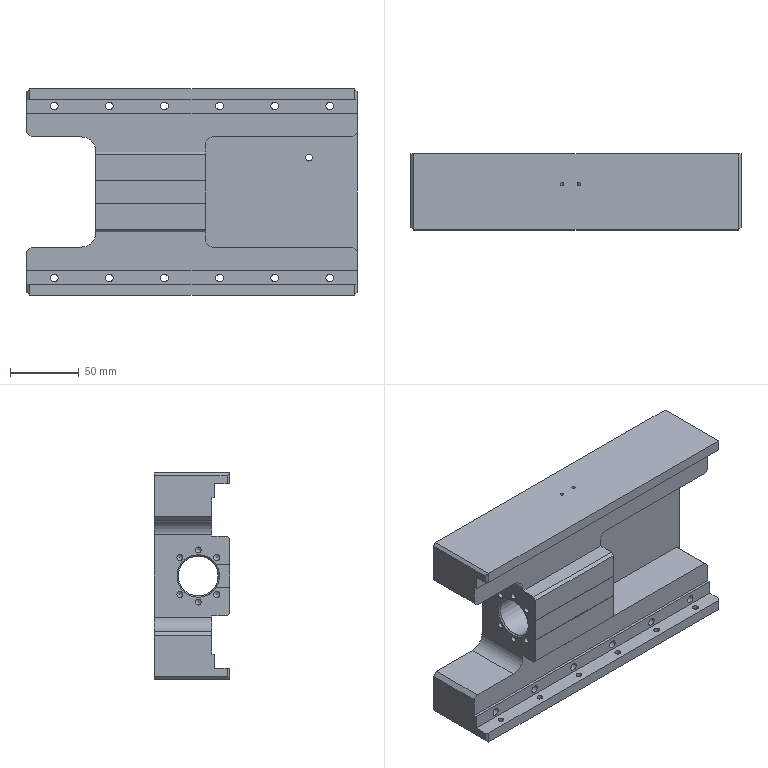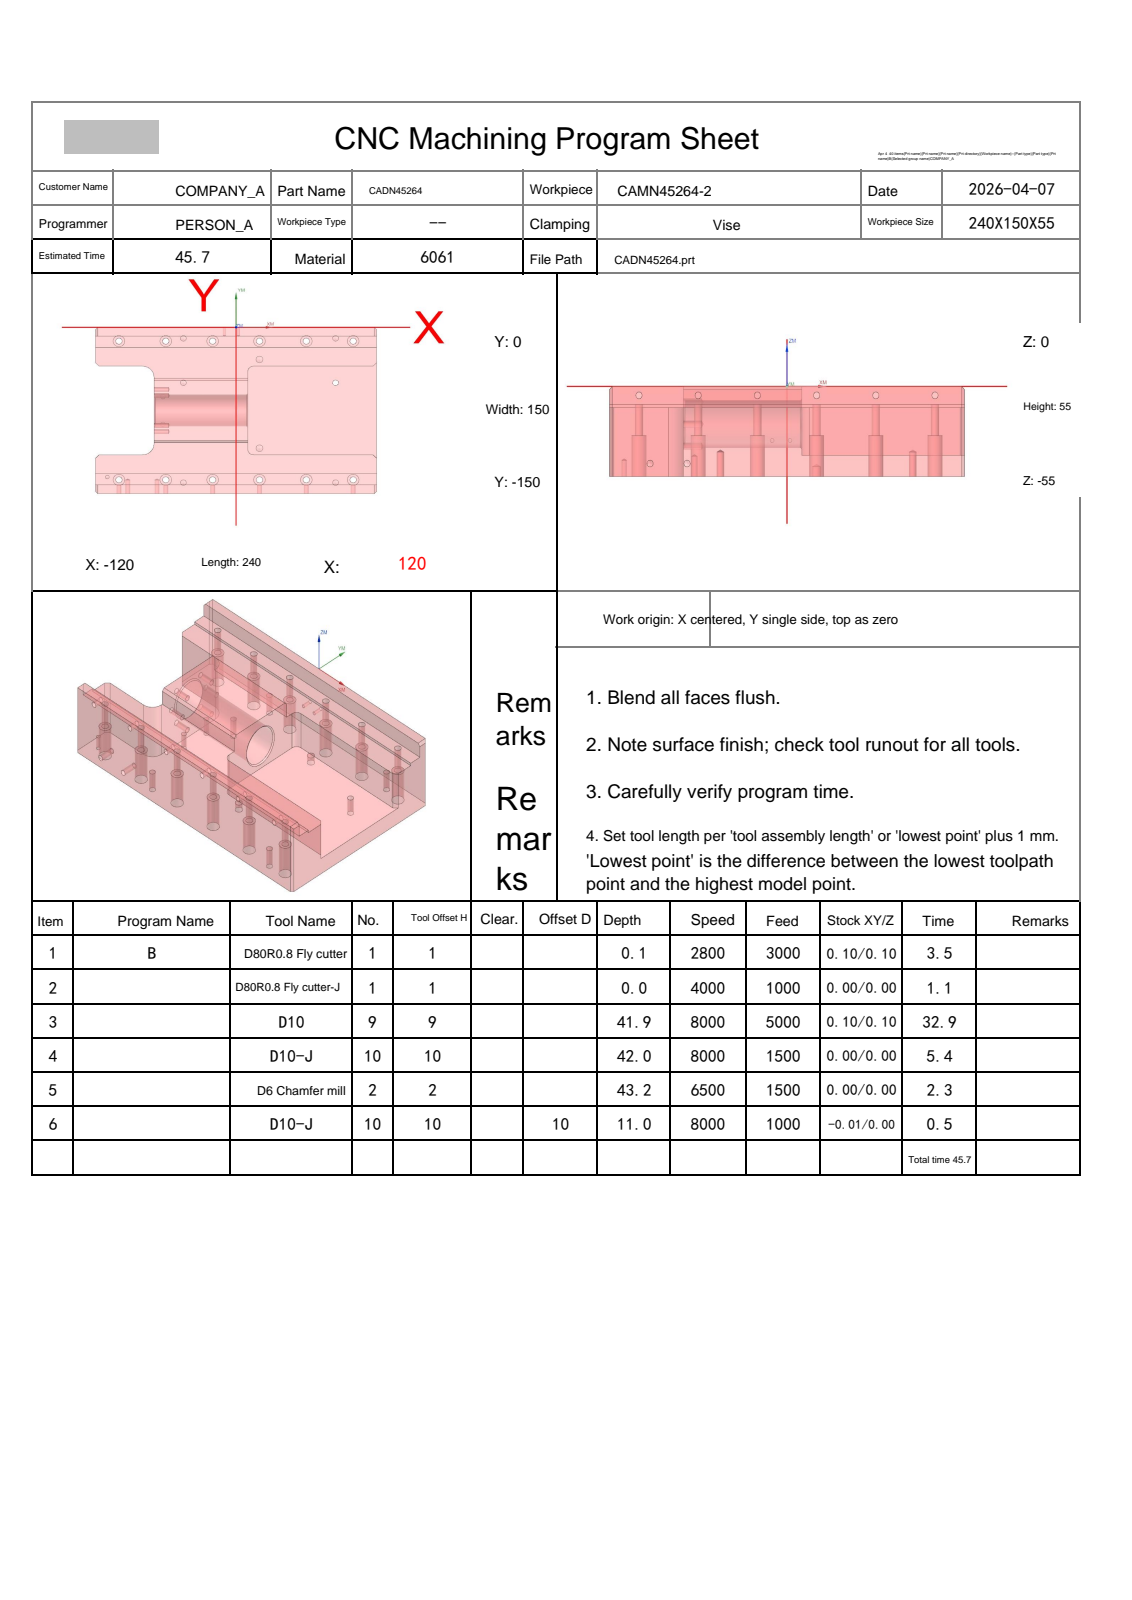NC program | NX | posted by the shop | part box 240 x 55 x 150 mm
Lines 209 to 1333 of 15848:
N3 T09 M06
(D10  D=10. R=0. H=09 ce=0.10 di=0.10)
G00 G90 G54 X134.5 Y-68. M03 S8000
G43 H09 Z14.5
M08
Z.626
G01 Z-.574 F5000.
X127.08
G03 X120.08 Y-75. I0.0 J-7.
G01 Y-110.836
X120.213 Y-110.937
X120.692 Y-111.365
X123. Y-113.672
Y-115.112
X120.08 Y-118.033
Y-126.698
Y-127.517
Y-136.418
Y-136.823
G02 X124.225 Y-139.047 I-.107 J-5.175
X125.085 Y-141.392 I-5.384 J-3.303
X125.115 Y-142. I-6.49 J-.629
G01 Y-148.068
X123.714 Y-149.47
X123.715 Y-142.
G03 X118.594 Y-136.9 I-5.121 J-.021
G01 X118.574
X-118.574
X-118.594
G03 X-123.715 Y-142. I0.0 J-5.121
G01 X-123.714 Y-149.467
X-125.115 Y-148.059
Y-141.994
G02 X-125.039 Y-141.028 I6.521 J-.026
X-123. Y-137.826 I5.116 J-1.008
X-120.08 Y-136.824 I3.077 J-4.21
G01 Y-136.418
Y-127.517
Y-126.698
Y-118.
X-120.057 Y-117.943
X-117.057 Y-114.943
X-117. Y-114.92
X-80.424
X-79.534 Y-114.909
X-78.648 Y-114.827
X-77.761 Y-114.664
X-76.874 Y-114.414
X-76.45 Y-114.263
X-75.989 Y-114.073
X-75.102 Y-113.626
X-74.43 Y-113.208
X-74.217 Y-113.06
X-73.329 Y-112.342
X-72.442 Y-111.425
X-72.102 Y-111.002
X-71.784 Y-110.56
X-71.556 Y-110.207
X-71.252 Y-109.677
X-70.925 Y-109.005
X-70.911 Y-108.936
X-70.845 Y-108.961
X-70.458 Y-108.999
X-70.082 Y-109.018
X-70.08 Y-107.714
X-65.641 Y-107.715
X10.
G03 X15.1 Y-102.574 I-.057 J5.157
G01 Y-47.426
G03 X10. Y-42.285 I-5.157 J-.015
G01 X-65.658
X-70.08 Y-42.286
X-70.082 Y-40.982
X-70.456 Y-41.001
X-70.826 Y-41.048
X-70.892 Y-41.075
X-70.907 Y-41.005
X-71.252 Y-40.323
X-71.556 Y-39.793
X-71.784 Y-39.441
X-72.457 Y-38.557
X-73.329 Y-37.658
X-74.217 Y-36.94
X-74.43 Y-36.792
X-75.101 Y-36.374
X-76.033 Y-35.908
X-76.875 Y-35.585
X-77.761 Y-35.336
X-78.648 Y-35.173
X-79.534 Y-35.091
X-80.424 Y-35.08
X-117.
X-117.057 Y-35.057
X-120.057 Y-32.057
X-120.08 Y-32.
Y-23.302
Y-22.483
Y-13.582
Y-13.176
G02 X-125.039 Y-8.972 I.157 J5.212
X-125.115 Y-8. I6.445 J.993
G01 Y-1.932
X-123.714 Y-.53
X-123.715 Y-8.
G03 X-118.594 Y-13.1 I5.121 J.021
G01 X-118.574
X118.574
X118.594
G03 X123.715 Y-8. I0.0 J5.121
G01 X123.714 Y-.533
X125.115 Y-1.941
Y-8.006
G02 X125.04 Y-8.965 I-6.521 J.026
X120.08 Y-13.176 I-5.118 J1.002
G01 Y-13.582
Y-22.483
Y-23.302
Y-31.967
X123. Y-34.888
Y-36.328
X120.69 Y-38.637
X120.356 Y-38.947
X120.08 Y-39.164
Y-71.986
G02 X119.662 Y-72.799 I-1. J0.0
G01 X113.498 Y-77.201
G03 X113.08 Y-78.014 I.582 J-.813
G01 Y-110.836
G03 X113.83 Y-113.987 I7. J0.0
G02 X113.935 Y-114.434 I-.894 J-.447
X113.83 Y-114.881 I-1. J0.0
G03 X113.08 Y-118.033 I6.25 J-3.152
G01 Y-126.696
Y-127.516
Y-128.903
G02 X112.083 Y-129.9 I-1. J.003
G01 X-71.13
G02 X-71.83 Y-129.613 I0.0 J1.
G01 X-73.319 Y-128.152
G03 X-73.767 Y-127.898 I-.7 J-.714
G02 X-75.638 Y-125.478 I.629 J2.42
X-73.741 Y-123.052 I2.5 J0.0
G01 X-66.347 Y-121.217
G02 X-65.745 Y-121.143 I.602 J-2.426
X-63.245 Y-123.643 I0.0 J-2.5
X-65.143 Y-126.07 I-2.5 J0.0
G01 X-71.264 Y-127.589
G03 X-71.774 Y-127.899 I.241 J-.971
G01 X-73.235 Y-129.56
G02 X-73.986 Y-129.9 I-.751 J.66
G01 X-112.083
G02 X-113.08 Y-128.903 I.003 J1.
G01 Y-127.516
Y-126.696
Y-122.917
G02 X-112.083 Y-121.92 I1. J-.003
G01 X-80.381
X-79.17 Y-121.905
X-77.69 Y-121.769
X-76.176 Y-121.49
X-74.746 Y-121.088
X-73.936 Y-120.798
X-73.077 Y-120.444
X-71.673 Y-119.737
X-70.576 Y-119.055
X-70.007 Y-118.658
X-68.595 Y-117.516
X-67.188 Y-116.061
X-66.526 Y-115.239
X-66.448 Y-115.129
G02 X-65.641 Y-114.715 I.811 J-.586
G01 X10.039
G03 X22.1 Y-102.584 I-.096 J12.157
G01 Y-47.416
G03 X10.039 Y-35.285 I-12.157 J-.026
G01 X-65.658
G02 X-66.448 Y-34.893 I.003 J1.
G01 X-67.141 Y-33.984
X-68.599 Y-32.481
X-70.007 Y-31.342
X-70.576 Y-30.945
X-71.68 Y-30.259
X-73.207 Y-29.494
X-74.67 Y-28.934
X-76.176 Y-28.51
X-77.69 Y-28.231
X-79.17 Y-28.095
X-80.381 Y-28.08
X-112.083
G02 X-113.08 Y-27.083 I.003 J1.
G01 Y-23.304
Y-22.484
Y-21.097
G02 X-112.083 Y-20.1 I1. J-.003
G01 X-73.995
G02 X-73.244 Y-20.44 I0.0 J-1.
G01 X-71.782 Y-22.101
G03 X-71.272 Y-22.412 I.751 J.66
G01 X-65.144 Y-23.929
G02 X-63.245 Y-26.355 I-.601 J-2.427
X-65.745 Y-28.855 I-2.5 J0.0
X-66.345 Y-28.782 I0.0 J2.5
G01 X-73.746 Y-26.95
G02 X-75.645 Y-24.523 I.601 J2.427
X-73.776 Y-22.104 I2.5 J0.0
G03 X-73.328 Y-21.85 I-.252 J.968
G01 X-71.838 Y-20.387
G02 X-71.137 Y-20.1 I.701 J-.713
G01 X112.083
G02 X113.08 Y-21.097 I-.003 J-1.
G01 Y-22.484
Y-23.304
Y-31.967
G03 X113.829 Y-35.118 I7. J0.0
G02 X113.935 Y-35.565 I-.895 J-.447
X113.829 Y-36.012 I-1. J0.0
G03 X113.08 Y-39.164 I6.251 J-3.151
G01 Y-71.986
G02 X112.662 Y-72.799 I-1. J0.0
G01 X106.498 Y-77.201
G03 X106.08 Y-78.014 I.582 J-.813
G01 Y-110.836
G03 X106.49 Y-114.198 I14. J0.0
G02 X106.518 Y-114.434 I-.972 J-.236
X106.49 Y-114.671 I-1. J0.0
G03 X106.08 Y-118.033 I13.59 J-3.362
G01 Y-121.904
G02 X105.084 Y-122.9 I-1. J.004
G01 X28.712
G02 X28.047 Y-122.647 I0.0 J1.
G01 X26.93 Y-121.653
G03 X26.311 Y-121.401 I-.664 J-.747
G02 X23.923 Y-118.904 I.112 J2.497
X25.377 Y-116.633 I2.5 J0.0
G01 X30.003 Y-114.503
G02 X31.049 Y-114.274 I1.046 J-2.271
X33.549 Y-116.774 I0.0 J-2.5
X32.095 Y-119.044 I-2.5 J0.0
G01 X28.471 Y-120.713
G03 X28.104 Y-121.002 I.418 J-.908
G01 X26.907 Y-122.519
G02 X26.122 Y-122.9 I-.785 J.619
G01 X-62.888
G02 X-63.385 Y-122.4 I.003 J.5
X-63.246 Y-122.054 I.5 J0.0
G01 X-63.063 Y-121.865
G02 X-62.709 Y-121.715 I.357 J-.35
G01 X10.066
G03 X29.1 Y-102.591 I-.123 J19.157
G01 Y-47.409
G03 X10.066 Y-28.285 I-19.157 J-.033
G01 X-62.708
G02 X-63.062 Y-28.135 I.003 J.5
G01 X-63.246 Y-27.946
G02 X-63.385 Y-27.6 I.361 J.346
X-62.887 Y-27.1 I.5 J0.0
G01 X26.122
G02 X26.907 Y-27.481 I0.0 J-1.
G01 X28.104 Y-28.998
G03 X28.47 Y-29.286 I.785 J.62
G01 X32.095 Y-30.956
G02 X33.549 Y-33.226 I-1.046 J-2.271
X31.049 Y-35.726 I-2.5 J0.0
X30.003 Y-35.497 I0.0 J2.5
G01 X25.377 Y-33.367
G02 X23.923 Y-31.096 I1.046 J2.271
X26.311 Y-28.599 I2.5 J0.0
G03 X26.93 Y-28.347 I-.045 J.999
G01 X28.047 Y-27.353
G02 X28.712 Y-27.1 I.665 J-.747
G01 X105.084
G02 X106.08 Y-28.096 I-.004 J-1.
G01 Y-31.967
G03 X106.49 Y-35.329 I14. J0.0
G02 X106.518 Y-35.565 I-.972 J-.236
X106.49 Y-35.801 I-1. J0.0
G03 X106.08 Y-39.164 I13.59 J-3.362
G01 Y-71.986
G02 X105.662 Y-72.799 I-1. J0.0
G01 X99.498 Y-77.201
G03 X99.08 Y-78.014 I.582 J-.813
G01 Y-110.836
G03 X99.364 Y-114.275 I21. J0.0
G01 X99.376 Y-114.434
X99.364 Y-114.594
G03 X99.293 Y-115.047 I20.716 J-3.439
G02 X98.309 Y-115.9 I-.989 J.147
G01 X34.129
G02 X33.134 Y-114.9 I.005 J1.
X33.241 Y-114.45 I1. J0.0
G03 X36.1 Y-102.597 I-23.298 J11.891
G01 Y-47.403
G03 X33.241 Y-35.55 I-26.157 J-.039
G02 X33.134 Y-35.1 I.893 J.45
X34.129 Y-34.1 I1. J0.0
G01 X98.309
G02 X99.293 Y-34.953 I-.005 J-1.
G03 X99.364 Y-35.406 I20.787 J2.986
G01 X99.376 Y-35.565
X99.364 Y-35.724
G03 X99.08 Y-39.164 I20.716 J-3.439
G01 Y-71.986
G02 X98.662 Y-72.799 I-1. J0.0
G01 X92.498 Y-77.201
G03 X92.08 Y-78.014 I.582 J-.813
G01 Y-107.905
G02 X91.085 Y-108.9 I-1. J.005
G01 X43.675
G02 X42.68 Y-107.9 I.005 J1.
G01 X42.691 Y-107.748
G03 X43.1 Y-102.603 I-32.748 J5.19
G01 Y-47.397
G03 X42.691 Y-42.252 I-33.157 J-.044
G01 X42.68 Y-42.1
G02 X43.675 Y-41.1 I1. J0.0
G01 X91.085
G02 X92.08 Y-42.095 I-.005 J-1.
G01 Y-71.986
G02 X91.662 Y-72.799 I-1. J0.0
G01 X85.498 Y-77.201
G03 X85.08 Y-78.014 I.582 J-.813
G01 Y-100.905
G02 X84.085 Y-101.9 I-1. J.005
G01 X51.095
G02 X50.1 Y-100.905 I.005 J1.
G01 Y-49.095
G02 X51.095 Y-48.1 I1. J-.005
G01 X84.085
G02 X85.08 Y-49.095 I-.005 J-1.
G01 Y-71.986
G02 X84.662 Y-72.799 I-1. J0.0
G01 X78.498 Y-77.201
G03 X78.08 Y-78.014 I.582 J-.813
G01 Y-93.905
G02 X77.085 Y-94.9 I-1. J.005
G01 X58.095
G02 X57.1 Y-93.905 I.005 J1.
G01 Y-56.095
G02 X58.095 Y-55.1 I1. J-.005
G01 X77.085
G02 X78.08 Y-56.095 I-.005 J-1.
G01 Y-71.986
G02 X77.662 Y-72.799 I-1. J0.0
G01 X71.498 Y-77.201
G03 X71.08 Y-78.014 I.582 J-.814
G01 Y-86.905
G02 X70.085 Y-87.9 I-1. J.005
G01 X65.095
G02 X64.1 Y-86.905 I.005 J1.
G01 Y-63.095
G02 X65.095 Y-62.1 I1. J-.005
G01 X70.085
G02 X71.08 Y-63.095 I-.005 J-1.
G01 Y-75.
Y-75.5
G03 X78.08 Y-82.5 I7. J0.0
G01 Z.626
G00 Z3.
G01 X134.5 Y-68. F6000.
G00 Z.053
G01 Z-1.147 F5000.
X127.08
G03 X120.08 Y-75. I0.0 J-7.
G01 Y-110.836
X120.213 Y-110.937
X120.692 Y-111.365
X123. Y-113.672
Y-115.112
X120.08 Y-118.033
Y-126.698
Y-127.517
Y-135.565
Y-136.418
Y-136.823
G02 X124.225 Y-139.047 I-.107 J-5.175
X125.158 Y-142.35 I-5.384 J-3.303
X125.151 Y-142.651 I-6.317 J0.0
G01 Y-148.
X125.127 Y-148.056
X124.287 Y-148.896
X124.289 Y-142.
G03 X119.158 Y-136.9 I-5.131 J-.031
G01 X119.147
X-119.147
X-119.158
G03 X-124.289 Y-142. I0.0 J-5.131
G01 X-124.287 Y-148.891
X-125.127 Y-148.046
X-125.151 Y-147.99
Y-142.647
X-125.13 Y-141.755
G02 X-120.08 Y-136.824 I5.207 J-.281
G01 Y-136.418
Y-135.565
Y-127.517
Y-126.698
Y-118.
X-120.057 Y-117.943
X-117.057 Y-114.943
X-117. Y-114.92
X-80.424
X-79.534 Y-114.909
X-78.648 Y-114.827
X-77.761 Y-114.664
X-76.874 Y-114.414
X-76.45 Y-114.263
X-75.989 Y-114.073
X-75.102 Y-113.626
X-74.43 Y-113.208
X-74.217 Y-113.06
X-73.329 Y-112.342
X-72.442 Y-111.425
X-72.102 Y-111.002
X-71.784 Y-110.56
X-71.556 Y-110.207
X-71.252 Y-109.677
X-70.925 Y-109.005
X-70.911 Y-108.936
X-70.845 Y-108.961
X-70.458 Y-108.999
X-70.082 Y-109.018
X-70.081 Y-108.287
X-66.091 Y-108.289
X10.063
G03 X13.404 Y-106.978 I0.0 J4.915
X15.1 Y-103.147 I-3.602 J3.886
G01 Y-46.853
X15.052 Y-46.317
G03 X10.011 Y-41.711 I-5.041 J-.456
G01 X-66.096
X-70.081 Y-41.713
Y-41.489
X-70.082 Y-40.982
X-70.456 Y-41.001
X-70.826 Y-41.048
X-70.892 Y-41.075
X-70.907 Y-41.005
X-71.252 Y-40.323
X-71.556 Y-39.793
X-71.784 Y-39.441
X-72.457 Y-38.557
X-73.329 Y-37.658
X-74.217 Y-36.94
X-74.43 Y-36.792
X-75.101 Y-36.374
X-76.033 Y-35.908
X-76.875 Y-35.585
X-77.761 Y-35.336
X-78.648 Y-35.173
X-79.534 Y-35.091
X-80.424 Y-35.08
X-117.
X-117.057 Y-35.057
X-120.057 Y-32.057
X-120.08 Y-32.
Y-23.302
Y-22.483
Y-14.435
Y-13.582
Y-13.176
G02 X-125.13 Y-8.242 I.157 J5.212
G01 X-125.151 Y-6.461
Y-2.
X-125.127 Y-1.944
X-124.287 Y-1.104
X-124.289 Y-8.
G03 X-119.158 Y-13.1 I5.131 J.031
G01 X-119.147
X119.147
X119.158
G03 X124.289 Y-8. I0.0 J5.131
G01 X124.287 Y-1.109
X125.127 Y-1.954
X125.151 Y-2.01
Y-6.462
X125.13 Y-8.245
G02 X123. Y-12.174 I-5.208 J.282
X120.08 Y-13.176 I-3.078 J4.21
G01 Y-13.582
Y-14.435
Y-22.483
Y-23.302
Y-31.967
X123. Y-34.888
Y-36.328
X120.69 Y-38.637
X120.356 Y-38.947
X120.08 Y-39.164
Y-71.986
G02 X119.662 Y-72.799 I-1. J0.0
G01 X113.498 Y-77.201
G03 X113.08 Y-78.014 I.582 J-.813
G01 Y-110.836
G03 X113.83 Y-113.988 I7. J0.0
G02 X113.935 Y-114.434 I-.895 J-.447
X113.83 Y-114.881 I-1. J0.0
G03 X113.08 Y-118.033 I6.25 J-3.152
G01 Y-126.696
Y-127.516
Y-128.904
G02 X112.083 Y-129.9 I-1. J.004
G01 X-71.135
G02 X-71.836 Y-129.613 I0.0 J1.
G01 X-73.33 Y-128.144
G03 X-73.776 Y-127.89 I-.701 J-.713
G02 X-75.64 Y-125.472 I.636 J2.418
X-73.736 Y-123.044 I2.5 J0.0
G01 X-66.641 Y-121.303
G02 X-66.045 Y-121.231 I.596 J-2.428
X-63.545 Y-123.731 I0.0 J-2.5
X-65.449 Y-126.159 I-2.5 J0.0
G01 X-71.268 Y-127.587
G03 X-71.78 Y-127.897 I.238 J-.971
G01 X-73.245 Y-129.561
G02 X-73.996 Y-129.9 I-.75 J.661
G01 X-112.083
G02 X-113.08 Y-128.904 I.004 J1.
G01 Y-127.516
Y-126.696
Y-122.916
G02 X-112.084 Y-121.92 I1. J-.004
G01 X-80.381
X-79.17 Y-121.905
X-77.69 Y-121.769
X-76.176 Y-121.49
X-74.746 Y-121.088
X-73.936 Y-120.798
X-73.077 Y-120.444
X-71.673 Y-119.737
X-70.576 Y-119.055
X-70.007 Y-118.658
X-68.59 Y-117.511
X-67.188 Y-116.061
X-66.864 Y-115.659
G02 X-66.091 Y-115.289 I.777 J-.629
G01 X10.063
G03 X18.163 Y-112.112 I0.0 J11.915
X22.1 Y-103.184 I-8.361 J9.019
G01 X22.023 Y-45.687
G03 X10.011 Y-34.711 I-12.012 J-1.086
G01 X-66.096
G02 X-66.885 Y-34.32 I.004 J1.
G01 X-67.141 Y-33.984
X-68.599 Y-32.481
X-70.007 Y-31.342
X-70.576 Y-30.945
X-71.68 Y-30.259
X-73.207 Y-29.494
X-74.67 Y-28.934
X-76.176 Y-28.51
X-77.69 Y-28.231
X-79.17 Y-28.095
X-80.381 Y-28.08
X-112.084
G02 X-113.08 Y-27.084 I.004 J1.
G01 Y-23.304
Y-22.484
Y-21.096
G02 X-112.083 Y-20.1 I1. J-.004
G01 X-74.005
G02 X-73.254 Y-20.439 I0.0 J-1.
G01 X-71.788 Y-22.103
G03 X-71.276 Y-22.414 I.75 J.661
G01 X-65.451 Y-23.839
G02 X-63.545 Y-26.268 I-.594 J-2.428
X-66.045 Y-28.768 I-2.5 J0.0
X-66.639 Y-28.696 I0.0 J2.5
G01 X-73.741 Y-26.958
G02 X-75.647 Y-24.529 I.594 J2.428
X-73.785 Y-22.112 I2.5 J0.0
G03 X-73.339 Y-21.858 I-.255 J.967
G01 X-71.844 Y-20.387
G02 X-71.143 Y-20.1 I.701 J-.713
G01 X112.083
G02 X113.08 Y-21.096 I-.004 J-1.
G01 Y-22.484
Y-23.304
Y-31.967
G03 X113.83 Y-35.119 I7. J0.0
G02 X113.935 Y-35.565 I-.895 J-.447
X113.83 Y-36.012 I-1. J0.0
G03 X113.08 Y-39.164 I6.25 J-3.152
G01 Y-71.986
G02 X112.662 Y-72.799 I-1. J0.0
G01 X106.498 Y-77.201
G03 X106.08 Y-78.014 I.582 J-.813
G01 Y-110.836
G03 X106.49 Y-114.198 I14. J0.0
G02 X106.518 Y-114.434 I-.972 J-.236
X106.49 Y-114.67 I-1. J0.0
G03 X106.08 Y-118.033 I13.59 J-3.363
G01 Y-121.904
G02 X105.084 Y-122.9 I-1. J.004
G01 X29.213
G02 X28.551 Y-122.649 I0.0 J1.
G01 X27.459 Y-121.684
G03 X26.827 Y-121.434 I-.662 J-.75
G02 X24.402 Y-118.935 I.075 J2.499
X25.824 Y-116.68 I2.5 J0.0
G01 X30.273 Y-114.553
G02 X31.351 Y-114.308 I1.078 J-2.255
X33.851 Y-116.808 I0.0 J-2.5
X32.43 Y-119.063 I-2.5 J0.0
G01 X28.963 Y-120.721
G03 X28.607 Y-121.007 I.431 J-.902
G01 X27.426 Y-122.516
G02 X26.638 Y-122.9 I-.788 J.616
G01 X-63.359
G02 X-63.657 Y-122.599 I.003 J.301
X-63.56 Y-122.379 I.301 J0.0
X-63.348 Y-122.289 I.214 J-.21
G01 X10.063
G03 X22.922 Y-117.245 I0.0 J18.915
X29.1 Y-103.205 I-13.121 J14.152
G01 X29.023 Y-45.366
G03 X10.013 Y-27.711 I-19.009 J-1.406
G01 X10.011
X-63.349
G02 X-63.574 Y-27.607 I.002 J.301
X-63.657 Y-27.4 I.217 J.207
X-63.36 Y-27.1 I.3 J0.0
G01 X26.653
G02 X27.441 Y-27.484 I0.0 J-1.
G01 X28.622 Y-28.994
G03 X28.978 Y-29.279 I.787 J.617
G01 X32.443 Y-30.934
G02 X33.866 Y-33.19 I-1.077 J-2.256
X31.366 Y-35.69 I-2.5 J0.0
X30.288 Y-35.446 I0.0 J2.5
G01 X25.84 Y-33.322
G02 X24.418 Y-31.066 I1.077 J2.256
X26.842 Y-28.567 I2.5 J0.0
G03 X27.473 Y-28.317 I-.03 J1.
G01 X28.566 Y-27.351
G02 X29.229 Y-27.1 I.662 J-.749
G01 X105.084
G02 X106.08 Y-28.096 I-.004 J-1.
G01 Y-31.967
G03 X106.49 Y-35.329 I14. J0.0
G02 X106.518 Y-35.565 I-.972 J-.236
X106.49 Y-35.801 I-1. J0.0
G03 X106.08 Y-39.164 I13.59 J-3.362
G01 Y-71.986
G02 X105.662 Y-72.799 I-1. J0.0
G01 X99.498 Y-77.201
G03 X99.08 Y-78.014 I.582 J-.813
G01 Y-110.836
G03 X99.364 Y-114.275 I21. J0.0
G01 X99.376 Y-114.434
X99.364 Y-114.593
G03 X99.293 Y-115.047 I20.716 J-3.44
G02 X98.309 Y-115.9 I-.989 J.147
G01 X34.41
G02 X33.415 Y-114.9 I.005 J1.
X33.511 Y-114.472 I1. J0.0
G03 X36.1 Y-103.221 I-23.709 J11.379
G01 X36.022 Y-45.103
G03 X33.524 Y-35.527 I-26.008 J-1.673
G02 X33.428 Y-35.1 I.904 J.427
X34.423 Y-34.1 I1. J0.0
G01 X98.309
G02 X99.293 Y-34.953 I-.005 J-1.
G03 X99.364 Y-35.406 I20.787 J2.986
G01 X99.376 Y-35.565
X99.364 Y-35.724
G03 X99.08 Y-39.164 I20.716 J-3.439
G01 Y-71.986
G02 X98.662 Y-72.799 I-1. J0.0
G01 X92.498 Y-77.201
G03 X92.08 Y-78.014 I.582 J-.813
G01 Y-107.905
G02 X91.085 Y-108.9 I-1. J.005
G01 X43.757
G02 X42.762 Y-107.9 I.005 J1.
G01 X42.771 Y-107.765
G03 X43.1 Y-103.233 I-32.969 J4.672
G01 X43.022 Y-44.873
X43.008 Y-44.653
G03 X42.762 Y-42.232 I-32.993 J-2.122
G01 X42.754 Y-42.1
G02 X43.749 Y-41.1 I1. J0.0
G01 X91.085
G02 X92.08 Y-42.095 I-.005 J-1.
G01 Y-71.986
G02 X91.662 Y-72.799 I-1. J0.0
G01 X85.498 Y-77.201
G03 X85.08 Y-78.014 I.582 J-.813
G01 Y-100.905
G02 X84.085 Y-101.9 I-1. J.005
G01 X51.092
G02 X50.097 Y-100.907 I.005 J1.
G01 X50.028 Y-49.096
G02 X51.023 Y-48.1 I1. J-.004
G01 X84.085
G02 X85.08 Y-49.095 I-.005 J-1.
G01 Y-71.986
G02 X84.662 Y-72.799 I-1. J0.0
G01 X78.498 Y-77.201
G03 X78.08 Y-78.014 I.582 J-.814
G01 Y-93.905
G02 X77.085 Y-94.9 I-1. J.005
G01 X58.082
G02 X57.088 Y-93.907 I.005 J1.
G01 X57.037 Y-56.096
G02 X58.032 Y-55.1 I1. J-.004
G01 X77.085
G02 X78.08 Y-56.095 I-.005 J-1.
G01 Y-71.986
G02 X77.662 Y-72.799 I-1. J0.0
G01 X71.498 Y-77.201
G03 X71.08 Y-78.014 I.582 J-.814
G01 Y-86.905
G02 X70.085 Y-87.9 I-1. J.005
G01 X65.073
G02 X64.078 Y-86.907 I.005 J1.
G01 X64.046 Y-63.096
G02 X65.041 Y-62.1 I1. J-.004
G01 X70.085
G02 X71.08 Y-63.095 I-.005 J-1.
G01 Y-75.
Y-75.5
G03 X78.08 Y-82.5 I7. J0.0
G01 Z.053
G00 Z3.
G01 X134.5 Y-68. F6000.
G00 Z-.521
G01 Z-1.721 F5000.
X127.08
G03 X120.08 Y-75. I0.0 J-7.
G01 Y-110.836
X120.213 Y-110.937
X120.692 Y-111.365
X123. Y-113.672
Y-115.112
X120.08 Y-118.033
Y-126.698
Y-127.517
Y-135.509
Y-136.418
Y-136.823
G02 X124.225 Y-139.047 I-.107 J-5.175
X125.158 Y-142.35 I-5.384 J-3.303
X125.151 Y-142.651 I-6.317 J0.0
G01 Y-148.
X125.127 Y-148.056
X124.86 Y-148.324
X124.862 Y-142.
G03 X119.742 Y-136.9 I-5.121 J-.021
G01 X119.721
X-119.721
X-119.742
G03 X-124.862 Y-142. I0.0 J-5.121
G01 X-124.86 Y-148.315
X-125.127 Y-148.046
X-125.151 Y-147.99
Y-142.647
X-125.13 Y-141.755
G02 X-120.08 Y-136.824 I5.207 J-.281
G01 Y-136.418
Y-135.509
Y-127.517
Y-126.698
Y-118.
X-120.057 Y-117.943
X-117.057 Y-114.943
X-117. Y-114.92
X-80.424
X-79.534 Y-114.909
X-78.648 Y-114.827
X-77.761 Y-114.664
X-76.874 Y-114.414
X-76.45 Y-114.263
X-75.989 Y-114.073
X-75.102 Y-113.626
X-74.43 Y-113.208
X-74.217 Y-113.06
X-73.329 Y-112.342
X-72.442 Y-111.425
X-72.102 Y-111.002
X-71.784 Y-110.56
X-71.556 Y-110.207
X-71.252 Y-109.677
X-70.925 Y-109.005
X-70.911 Y-108.936
X-70.845 Y-108.961
X-70.458 Y-108.999
X-70.082 Y-109.018
Y-108.861
X-66.575 Y-108.862
X10.
G03 X15.1 Y-103.742 I-.021 J5.121
G01 Y-103.721
Y-46.279
Y-46.258
G03 X10. Y-41.138 I-5.121 J0.0
G01 X-66.573
X-70.082 Y-41.139
X-70.085 Y-40.982
X-70.456 Y-41.001
X-70.826 Y-41.048
X-70.892 Y-41.075
X-70.907 Y-41.005
X-71.252 Y-40.323
X-71.556 Y-39.793
X-71.784 Y-39.441
X-72.457 Y-38.557
X-73.329 Y-37.658
X-74.217 Y-36.94
X-74.43 Y-36.792
X-75.101 Y-36.374
X-76.033 Y-35.908
X-76.875 Y-35.585
X-77.761 Y-35.336
X-78.648 Y-35.173
X-79.534 Y-35.091
X-80.424 Y-35.08
X-117.
X-117.057 Y-35.057
X-120.057 Y-32.057
X-120.08 Y-32.
Y-23.302
Y-22.483
Y-14.491
Y-13.582
Y-13.176
G02 X-123. Y-12.174 I.157 J5.212
X-125.13 Y-8.242 I3.077 J4.21
G01 X-125.151 Y-6.461
Y-2.
X-125.127 Y-1.944
X-124.86 Y-1.676
X-124.862 Y-8.
G03 X-119.742 Y-13.1 I5.121 J.021
G01 X-119.721
X119.721
X119.742
G03 X124.862 Y-8. I0.0 J5.121
G01 X124.86 Y-1.685
X125.127 Y-1.954
X125.151 Y-2.01
Y-6.462
X125.13 Y-8.245
G02 X120.08 Y-13.176 I-5.208 J.282
G01 Y-13.582
Y-14.491
Y-22.483
Y-23.302
Y-31.967
X123. Y-34.888
Y-36.328
X120.69 Y-38.637
X120.356 Y-38.947
X120.08 Y-39.164
Y-71.986
G02 X119.662 Y-72.799 I-1. J0.0
G01 X113.498 Y-77.201
G03 X113.08 Y-78.014 I.582 J-.813
G01 Y-110.836
G03 X113.83 Y-113.988 I7. J0.0
G02 X113.935 Y-114.434 I-.895 J-.447
X113.83 Y-114.881 I-1. J0.0
G03 X113.08 Y-118.033 I6.25 J-3.152
G01 Y-126.696
Y-127.516
Y-128.904
G02 X112.084 Y-129.9 I-1. J.004
G01 X-112.084
G02 X-113.08 Y-128.904 I.004 J1.
G01 Y-127.516
Y-126.696
Y-122.916
G02 X-112.084 Y-121.92 I1. J-.004
G01 X-80.381
X-79.17 Y-121.905
X-77.69 Y-121.769
X-76.176 Y-121.49
X-75.178 Y-121.209
G02 X-74.907 Y-121.172 I.271 J-.963
X-74.42 Y-121.298 I0.0 J-1.
G01 X-72.615 Y-122.305
G03 X-72.128 Y-122.432 I.487 J.873
G01 X-72.103
X10.844 Y-120.337
X10.907 Y-120.336
G02 X13.407 Y-122.836 I0.0 J-2.5
X10.97 Y-125.335 I-2.5 J0.0
G01 X-73.145 Y-127.46
X-73.208 Y-127.461
G02 X-75.708 Y-124.961 I0.0 J2.5
X-74.414 Y-122.77 I2.5 J0.0
G03 X-73.992 Y-122.322 I-.482 J.876
G01 X-73.257 Y-120.771
G02 X-72.803 Y-120.306 I.904 J-.428
G01 X-71.673 Y-119.737
X-70.576 Y-119.055
X-70.007 Y-118.658
X-68.595 Y-117.516
X-67.287 Y-116.164
G02 X-66.575 Y-115.862 I.716 J-.698
G01 X10.014
G03 X22.1 Y-103.742 I-.035 J12.121
G01 Y-103.71
Y-46.29
Y-46.258
G03 X10.014 Y-34.138 I-12.121 J0.0
G01 X-66.573
G02 X-67.284 Y-33.837 I.004 J1.
G01 X-68.599 Y-32.481
X-70.007 Y-31.342
X-70.576 Y-30.945
X-71.68 Y-30.259
X-72.783 Y-29.706
G02 X-73.235 Y-29.249 I.447 J.894
G01 X-74.003 Y-27.669
G03 X-74.42 Y-27.23 I-.899 J-.437
G02 X-75.715 Y-25.039 I1.205 J2.19
X-73.215 Y-22.539 I2.5 J0.0
G01 X-73.152 Y-22.54
X10.97 Y-24.665
G02 X13.407 Y-27.164 I-.063 J-2.499
X10.907 Y-29.664 I-2.5 J0.0
G01 X10.844 Y-29.663
X-72.102 Y-27.568
X-72.127
G03 X-72.618 Y-27.697 I0.0 J-1.
G01 X-74.405 Y-28.703
G02 X-74.895 Y-28.832 I-.49 J.871
X-75.165 Y-28.794 I0.0 J1.
G01 X-76.176 Y-28.51
X-77.69 Y-28.231
X-79.17 Y-28.095
X-80.381 Y-28.08
X-112.084
G02 X-113.08 Y-27.084 I.004 J1.
G01 Y-23.304
Y-22.484
Y-21.096
G02 X-112.084 Y-20.1 I1. J-.004
G01 X112.084
G02 X113.08 Y-21.096 I-.004 J-1.
G01 Y-22.484
Y-23.304
Y-31.967
G03 X113.83 Y-35.119 I7. J0.0
G02 X113.935 Y-35.565 I-.895 J-.446
X113.83 Y-36.012 I-1. J0.0
G03 X113.08 Y-39.164 I6.25 J-3.152
G01 Y-71.986
G02 X112.662 Y-72.799 I-1. J0.0
G01 X106.498 Y-77.201
G03 X106.08 Y-78.014 I.582 J-.813
G01 Y-110.836
G03 X106.49 Y-114.199 I14. J0.0
G02 X106.518 Y-114.434 I-.972 J-.236
X106.49 Y-114.67 I-1. J0.0
G03 X106.08 Y-118.033 I13.59 J-3.363
G01 Y-121.905
G02 X105.085 Y-122.9 I-1. J.004
G01 X13.702
G02 X13.504 Y-122.7 I.002 J.2
X13.664 Y-122.504 I.2 J0.0
G03 X29.1 Y-103.742 I-3.685 J18.762
G01 Y-103.702
Y-46.298
Y-46.258
G03 X13.664 Y-27.496 I-19.121 J0.0
G02 X13.504 Y-27.3 I.041 J.196
X13.702 Y-27.1 I.2 J0.0
G01 X105.085
G02 X106.08 Y-28.095 I-.005 J-1.
G01 Y-31.967
G03 X106.49 Y-35.33 I14. J0.0
G02 X106.518 Y-35.565 I-.972 J-.236
X106.49 Y-35.801 I-1. J0.0
G03 X106.08 Y-39.164 I13.59 J-3.363
G01 Y-71.986
G02 X105.662 Y-72.799 I-1. J0.0
G01 X99.498 Y-77.201
G03 X99.08 Y-78.014 I.582 J-.813
G01 Y-110.836
G03 X99.364 Y-114.276 I21. J0.0
G01 X99.376 Y-114.434
X99.364 Y-114.593
G03 X99.293 Y-115.047 I20.716 J-3.44
G02 X98.309 Y-115.9 I-.989 J.147
G01 X34.693
G02 X33.698 Y-114.9 I.005 J1.
X33.785 Y-114.493 I1. J0.0
G03 X36.1 Y-103.742 I-23.806 J10.751
G01 Y-103.695
Y-46.305
Y-46.258
G03 X33.785 Y-35.507 I-26.121 J0.0
G02 X33.698 Y-35.1 I.913 J.407
X34.693 Y-34.1 I1. J0.0
G01 X98.309
G02 X99.293 Y-34.953 I-.005 J-1.
G03 X99.364 Y-35.407 I20.787 J2.986
G01 X99.376 Y-35.565
X99.364 Y-35.724
G03 X99.08 Y-39.164 I20.716 J-3.44
G01 Y-71.986
G02 X98.662 Y-72.799 I-1. J0.0
G01 X92.498 Y-77.201
G03 X92.08 Y-78.014 I.582 J-.813
G01 Y-107.905
G02 X91.085 Y-108.9 I-1. J.005
G01 X43.841
G02 X42.846 Y-107.9 I.005 J1.
G01 X42.853 Y-107.783
G03 X43.1 Y-103.742 I-32.873 J4.041
G01 Y-103.689
Y-46.311
Y-46.258
G03 X42.853 Y-42.217 I-33.121 J0.0
G01 X42.846 Y-42.1
G02 X43.841 Y-41.1 I1. J0.0
G01 X91.085
G02 X92.08 Y-42.095 I-.005 J-1.
G01 Y-71.986
G02 X91.662 Y-72.799 I-1. J0.0
G01 X85.498 Y-77.201
G03 X85.08 Y-78.014 I.582 J-.813
G01 Y-100.905
G02 X84.085 Y-101.9 I-1. J.005
G01 X51.095
G02 X50.1 Y-100.905 I.005 J1.
G01 Y-49.095
G02 X51.095 Y-48.1 I1. J-.005
G01 X84.085
G02 X85.08 Y-49.095 I-.005 J-1.
G01 Y-71.986
G02 X84.662 Y-72.799 I-1. J0.0
G01 X78.498 Y-77.201
G03 X78.08 Y-78.014 I.582 J-.814
G01 Y-93.905
G02 X77.085 Y-94.9 I-1. J.005
G01 X58.095
G02 X57.1 Y-93.905 I.005 J1.
G01 Y-56.095
G02 X58.095 Y-55.1 I1. J-.005
G01 X77.085
G02 X78.08 Y-56.095 I-.005 J-1.
G01 Y-71.986
G02 X77.662 Y-72.799 I-1. J0.0
G01 X71.498 Y-77.201
G03 X71.08 Y-78.014 I.582 J-.814
G01 Y-86.906
G02 X70.086 Y-87.9 I-1. J.006
G01 X65.094
G02 X64.1 Y-86.906 I.006 J1.
G01 Y-63.094
G02 X65.094 Y-62.1 I1. J-.006
G01 X70.086
G02 X71.08 Y-63.094 I-.006 J-1.
G01 Y-75.
Y-75.5
G03 X78.08 Y-82.5 I7. J0.0
G01 Z-.521
G00 Z3.
G01 X134.5 Y-68. F6000.
G00 Z-1.095
G01 Z-2.295 F5000.
X127.08
G03 X120.08 Y-75. I0.0 J-7.
G01 Y-110.836
X120.213 Y-110.937
X120.692 Y-111.365
X123. Y-113.672
Y-115.112
X120.08 Y-118.033
Y-126.698
Y-127.517
Y-136.418
Y-136.823
G02 X124.225 Y-139.047 I-.107 J-5.175
X125.158 Y-142.35 I-5.384 J-3.303
X125.151 Y-142.651 I-6.317 J0.0
G01 Y-148.
X125.127 Y-148.056
X125.099 Y-148.084
X125.1 Y-142.
X125.099 Y-141.878
G03 X120. Y-136.9 I-5.099 J-.122
G01 X-120.
G03 X-125.098 Y-141.851 I0.0 J-5.1
G01 X-125.1 Y-142.
X-125.099 Y-148.074
X-125.127 Y-148.046
X-125.151 Y-147.99
Y-142.647
X-125.13 Y-141.755
G02 X-120.08 Y-136.824 I5.207 J-.281
G01 Y-136.418
Y-127.517
Y-126.698
Y-118.
X-120.057 Y-117.943
X-117.057 Y-114.943
X-117. Y-114.92
X-80.424
X-79.534 Y-114.909
X-78.648 Y-114.827
X-77.761 Y-114.664
X-76.874 Y-114.414
X-76.45 Y-114.263
X-75.989 Y-114.073
X-75.102 Y-113.626
X-74.43 Y-113.208
X-74.217 Y-113.06
X-73.329 Y-112.342
X-72.442 Y-111.425
X-72.102 Y-111.002
X-71.784 Y-110.56
X-71.556 Y-110.207
X-71.252 Y-109.677
X-70.929 Y-109.015
G03 X-70. Y-109.1 I.929 J5.015
G01 X10.
G03 X15.1 Y-104. I0.0 J5.1
G01 Y-45.999
G03 X10. Y-40.9 I-5.1 J-.001
G01 X-70.
G03 X-70.918 Y-40.983 I0.0 J-5.1
G01 X-71.252 Y-40.323